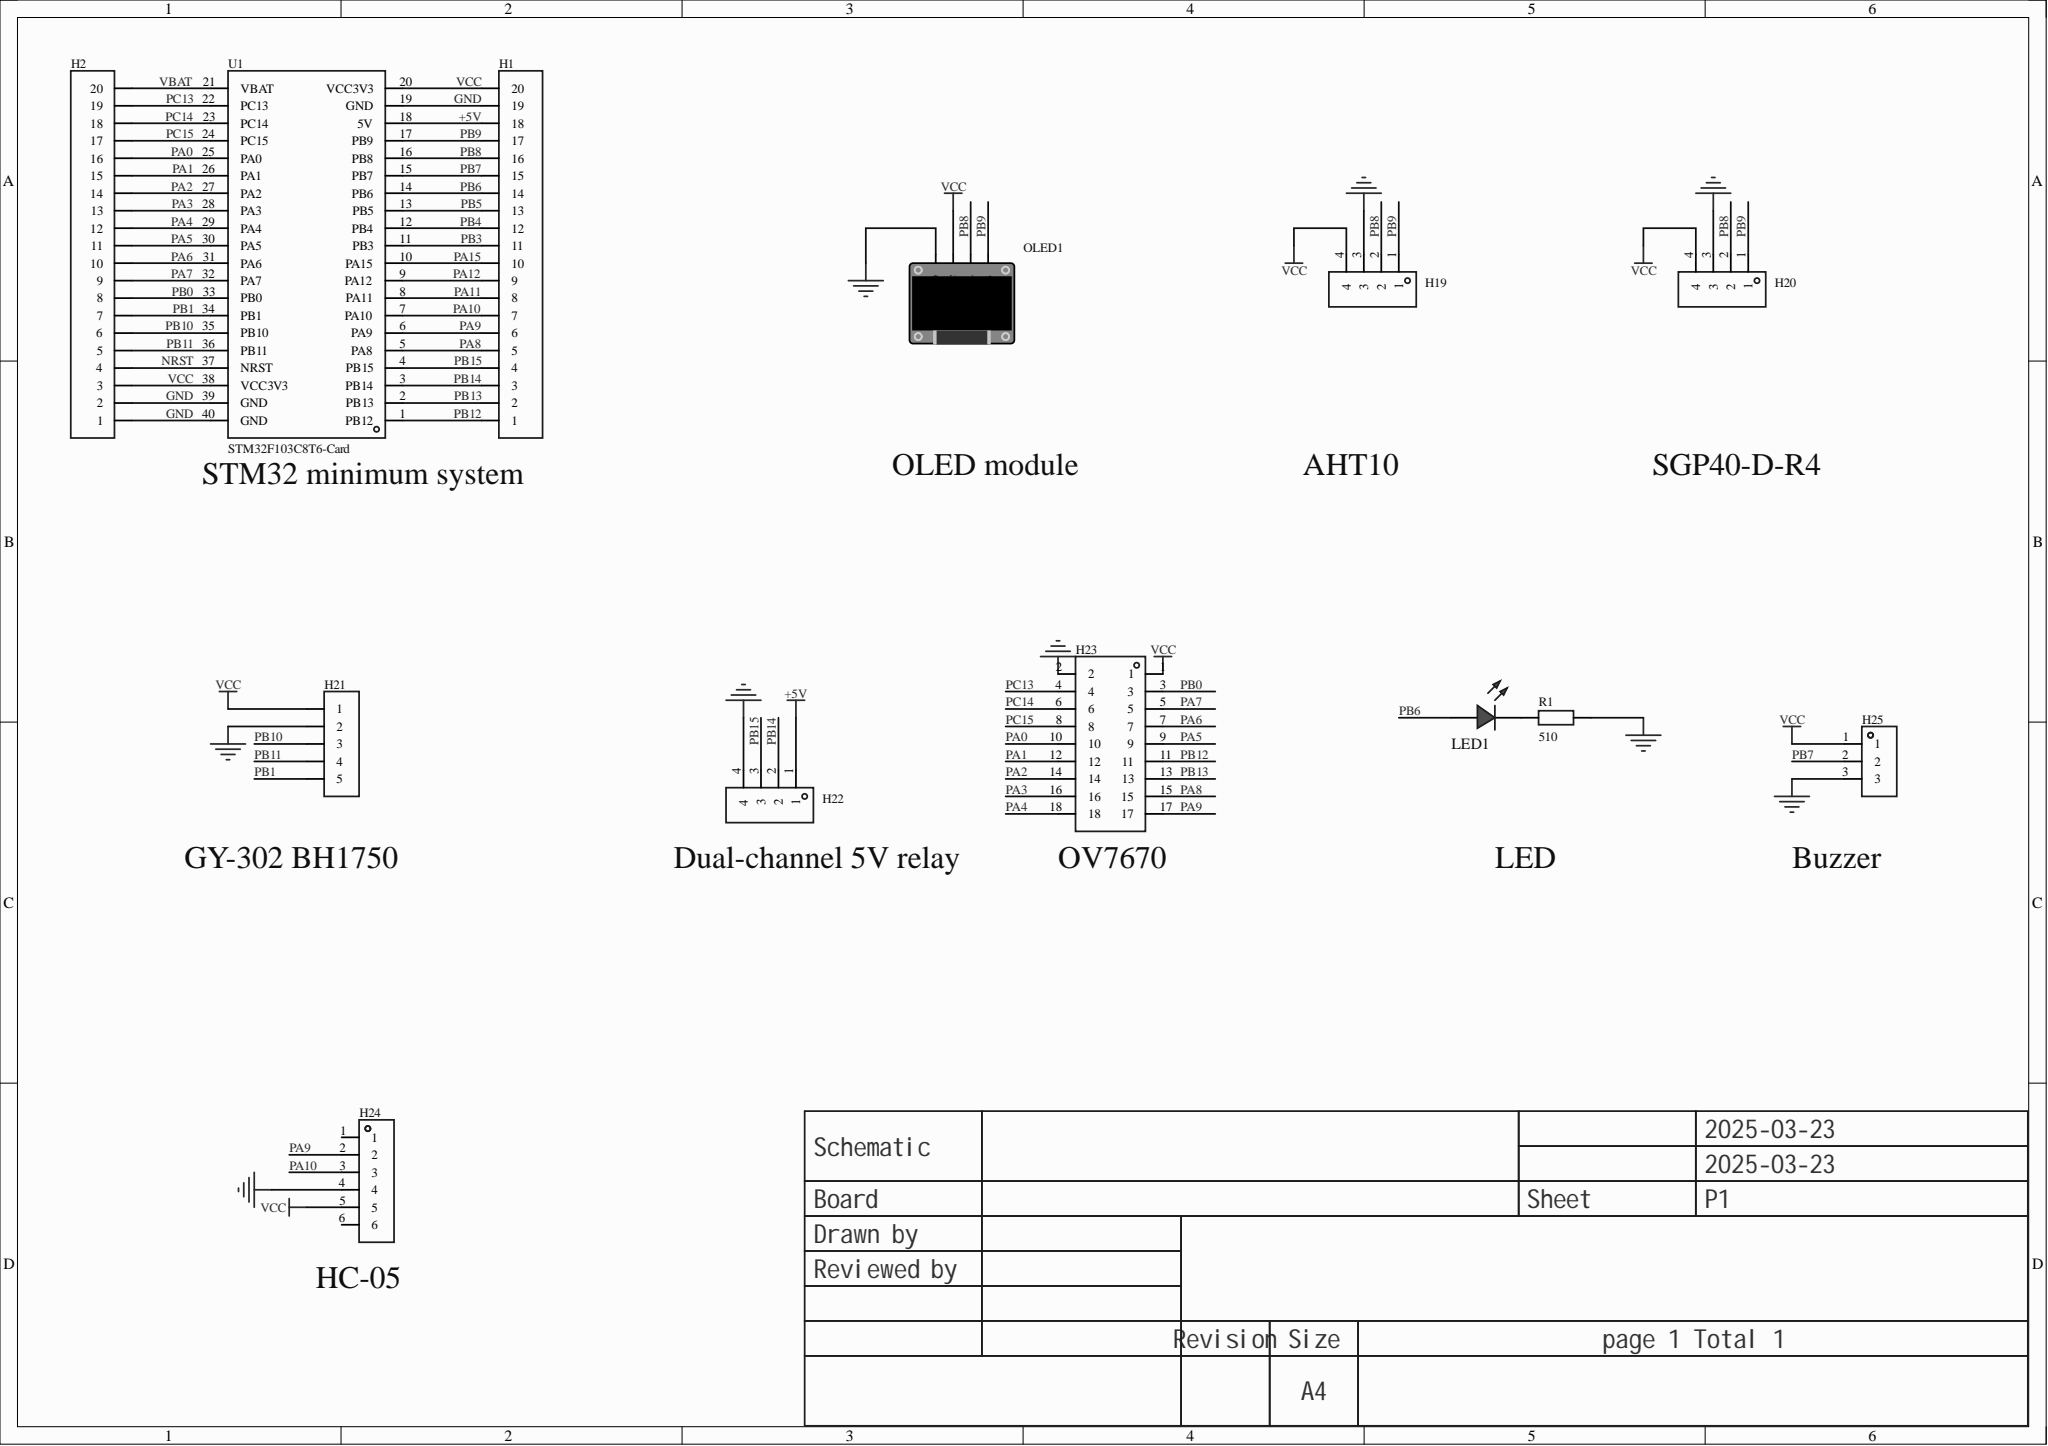Circuit board | Altium Designer | 13 parts | 38 nets
Bill of materials:
Comment,Description,Designator,Footprint,LibRef,Quantity
"","","H1, H2","HDR-TH_20P-P2.54-V-F","HDR-F_2.54_1x20P","2"
"","","H19, H20, H22","HDR-TH_4P-P2.54-V-F","HDR-F_2.54_1x4P","3"
"","","H21","HDR-TH_5P-P2.54-V-F","HDR-F_2.54_1x5P","1"
"","","H23","HDR-TH_18P-P2.54-V-M-R2-C9-S2.54","HDR-M_2.54_2x9","1"
"","","H24","HDR-TH_6P-P2.54-V-F","HDR-F_2.54_1x6P","1"
"","","H25","HDR-TH_3P-P2.54-V-F","HDR-F_2.54_1x3P","1"
"","","LED1","LED_0603","LED_0603-R","1"
"","","OLED1","0.96OLED_4P","0.96OLED模块_4P","1"
"510","","R1","R0603","Res_0603","1"
"STM32F103C8T6-Card","","U1","CONN-TH_L53.3-W22.9_STM32F103C8T6-CARD","STM32F103C8T6-Card","1"
Netlist (Protel format):
[
H1
HDR-TH_20P-P2.54-V-F




]
[
H2
HDR-TH_20P-P2.54-V-F




]
[
H19
HDR-TH_4P-P2.54-V-F




]
[
H20
HDR-TH_4P-P2.54-V-F




]
[
H21
HDR-TH_5P-P2.54-V-F




]
[
H22
HDR-TH_4P-P2.54-V-F




]
[
H23
HDR-TH_18P-P2.54-V-M-R2-C9-S2.54




]
[
H24
HDR-TH_6P-P2.54-V-F




]
[
H25
HDR-TH_3P-P2.54-V-F




]
[
LED1
LED_0603




]
[
OLED1
0.96OLED_4P




]
[
R1
R0603
510



]
[
U1
CONN-TH_L53.3-W22.9_STM32F103C8T6-CARD
STM32F103C8T6-Card



]
(
VCC
H1-20
H2-3
H19-4
H20-4
H21-1
H23-1
H24-5
H25-1
OLED1-2
U1-20
U1-38
)
(
VBAT
H2-20
U1-21
)
(
PC15
H2-17
H23-8
U1-24
)
(
PC14
H2-18
H23-6
U1-23
)
(
PC13
H2-19
H23-4
U1-22
)
(
PB15
H1-4
H22-3
U1-4
)
(
PB14
H1-3
H22-2
U1-3
)
(
PB13
H1-2
H23-13
U1-2
)
(
PB12
H1-1
H23-11
U1-1
)
(
PB11
H2-5
H21-4
U1-36
)
(
PB10
H2-6
H21-3
U1-35
)
(
PB9
H1-17
H19-1
H20-1
OLED1-4
U1-17
)
(
PB8
H1-16
H19-2
H20-2
OLED1-3
U1-16
)
(
PB7
H1-15
H25-2
U1-15
)
(
PB6
H1-14
LED1-2
U1-14
)
(
PB5
H1-13
U1-13
)
(
PB4
H1-12
U1-12
)
(
PB3
H1-11
U1-11
)
(
PB1
H2-7
H21-5
U1-34
)
(
PB0
H2-8
H23-3
U1-33
)
(
PA15
H1-10
U1-10
)
(
PA12
H1-9
U1-9
)
(
PA11
H1-8
U1-8
)
(
PA10
H1-7
H24-3
U1-7
)
(
PA9
H1-6
H23-17
H24-2
U1-6
)
(
PA8
H1-5
H23-15
U1-5
)
(
PA7
H2-9
H23-5
U1-32
)
(
PA6
H2-10
H23-7
U1-31
)
(
PA5
H2-11
H23-9
U1-30
)
(
PA4
H2-12
H23-18
U1-29
)
(
PA3
H2-13
H23-16
U1-28
)
(
PA2
H2-14
H23-14
U1-27
)
(
PA1
H2-15
H23-12
U1-26
)
(
PA0
H2-16
H23-10
U1-25
)
(
NRST
H2-4
U1-37
)
(
NetLED1_1
LED1-1
R1-1
)
(
GND
H1-19
H2-1
H2-2
H19-3
H20-3
H21-2
H22-4
H23-2
H24-4
H25-3
OLED1-1
R1-2
U1-19
U1-39
U1-40
)
(
+5V
H1-18
H22-1
U1-18
)